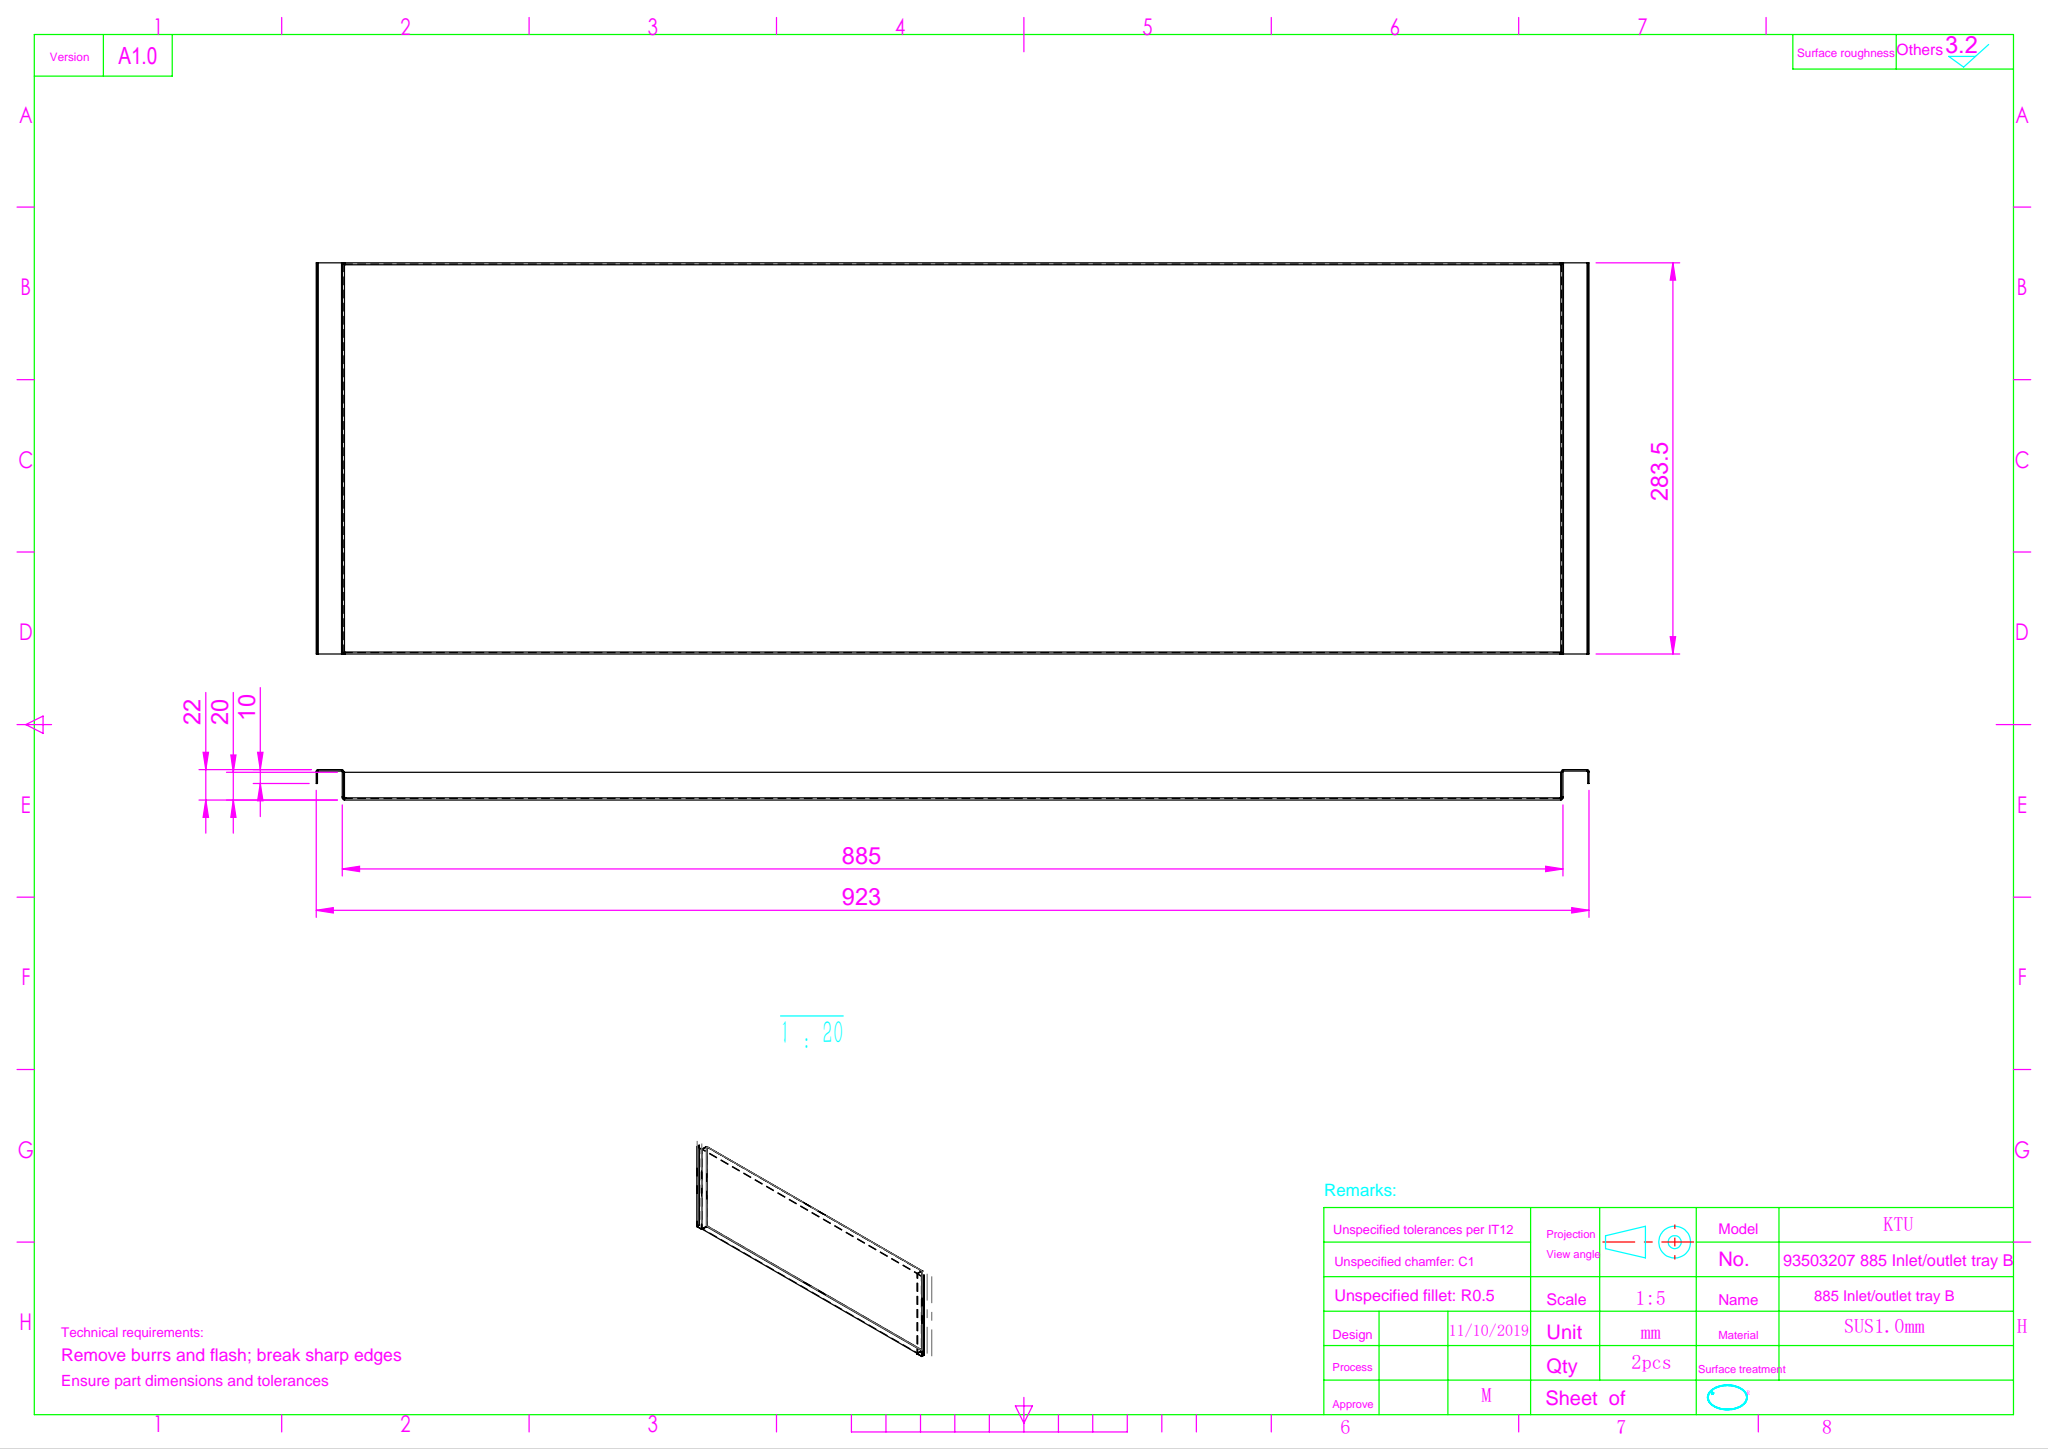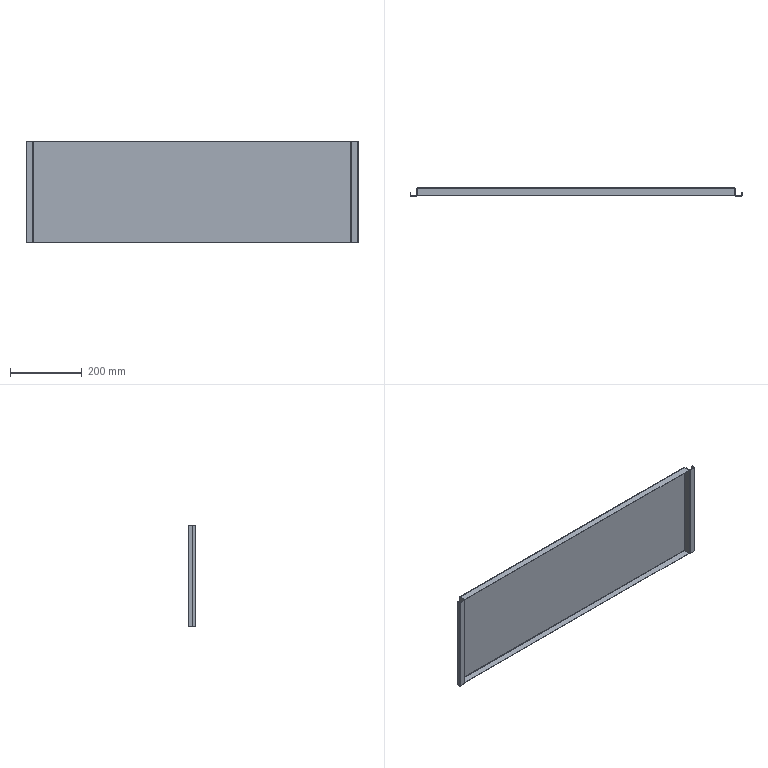Part | SolidWorks | features CornerRelief 1, EdgeFlange 1, FlatPattern 1, SMBaseFlange 1, SheetMetal 1 | 1 solid | 82 faces | box 923 x 22 x 283.5 mm | volume 310702 mm3 | plane 50 | cylinder 20 | spline 12 | commonest cylinder face diameters 1 x12 3 x8